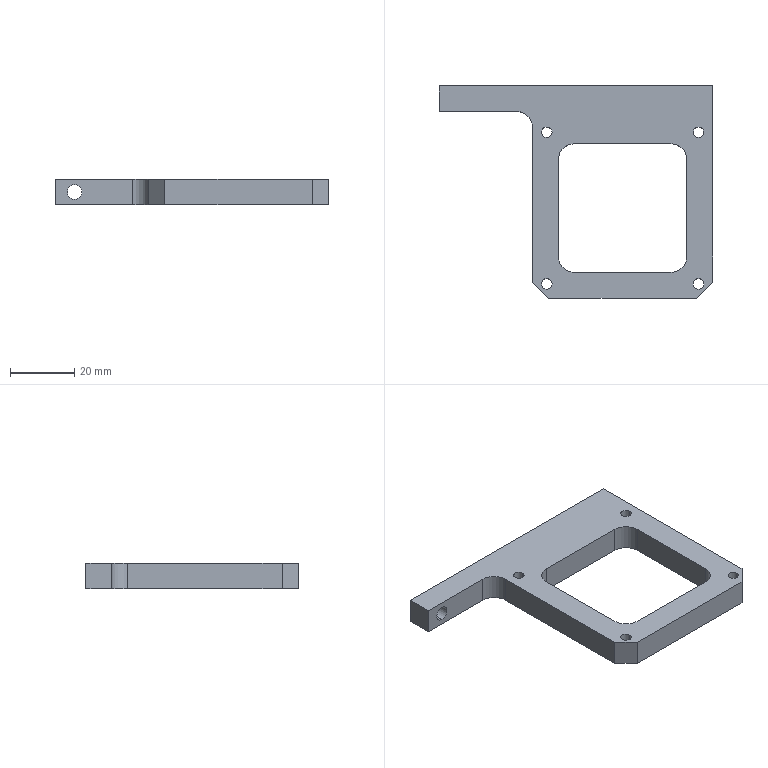Part | SolidWorks | features BaseBody 1 | 1 solid | 33 faces | box 85 x 66 x 8 mm | volume 18162 mm3 | cylinder 17 | plane 14 | cone 2 | commonest cylinder face diameters 3.242 x10 10 x5 4.5 x2
STEP:
#1=CARTESIAN_POINT('',(-10.691,18.57,0.));
#2=VERTEX_POINT('',#1);
#3=CARTESIAN_POINT('',(-7.449,18.57,0.));
#4=VERTEX_POINT('',#3);
#5=CARTESIAN_POINT('',(-9.07,18.57,0.));
#6=DIRECTION('',(0.,0.,1.));
#7=DIRECTION('',(1.,0.,0.));
#8=AXIS2_PLACEMENT_3D('',#5,#6,#7);
#9=CIRCLE('',#8,1.621);
#10=EDGE_CURVE('',#2,#4,#9,.T.);
#11=ORIENTED_EDGE('',*,*,#10,.F.);
#12=CARTESIAN_POINT('',(-10.691,18.57,8.));
#13=VERTEX_POINT('',#12);
#14=CARTESIAN_POINT('',(-10.691,18.57,-99.912));
#15=DIRECTION('',(0.,0.,1.));
#16=VECTOR('',#15,1000.);
#17=LINE('',#14,#16);
#18=EDGE_CURVE('',#2,#13,#17,.T.);
#19=ORIENTED_EDGE('',*,*,#18,.T.);
#20=CARTESIAN_POINT('',(-7.449,18.57,8.));
#21=VERTEX_POINT('',#20);
#22=CARTESIAN_POINT('',(-9.07,18.57,8.));
#23=DIRECTION('',(0.,0.,-1.));
#24=DIRECTION('',(1.,0.,0.));
#25=AXIS2_PLACEMENT_3D('',#22,#23,#24);
#26=CIRCLE('',#25,1.621);
#27=EDGE_CURVE('',#21,#13,#26,.T.);
#28=ORIENTED_EDGE('',*,*,#27,.F.);
#29=CARTESIAN_POINT('',(-7.449,18.57,-99.912));
#30=DIRECTION('',(0.,0.,1.));
#31=VECTOR('',#30,1000.);
#32=LINE('',#29,#31);
#33=EDGE_CURVE('',#4,#21,#32,.T.);
#34=ORIENTED_EDGE('',*,*,#33,.F.);
#35=EDGE_LOOP('',(#11,#19,#28,#34));
#36=FACE_OUTER_BOUND('',#35,.T.);
#37=CARTESIAN_POINT('',(-9.07,18.57,-99.912));
#38=DIRECTION('',(0.,0.,1.));
#39=DIRECTION('',(1.,0.,0.));
#40=AXIS2_PLACEMENT_3D('',#37,#38,#39);
#41=CYLINDRICAL_SURFACE('',#40,1.621);
#42=ADVANCED_FACE('',(#36),#41,.F.);
#43=CARTESIAN_POINT('',(36.449,18.57,0.));
#44=VERTEX_POINT('',#43);
#45=CARTESIAN_POINT('',(39.691,18.57,0.));
#46=VERTEX_POINT('',#45);
#47=CARTESIAN_POINT('',(38.07,18.57,0.));
#48=DIRECTION('',(0.,0.,1.));
#49=DIRECTION('',(1.,0.,0.));
#50=AXIS2_PLACEMENT_3D('',#47,#48,#49);
#51=CIRCLE('',#50,1.621);
#52=EDGE_CURVE('',#44,#46,#51,.T.);
#53=ORIENTED_EDGE('',*,*,#52,.F.);
#54=CARTESIAN_POINT('',(36.449,18.57,8.));
#55=VERTEX_POINT('',#54);
#56=CARTESIAN_POINT('',(36.449,18.57,-99.912));
#57=DIRECTION('',(0.,0.,1.));
#58=VECTOR('',#57,1000.);
#59=LINE('',#56,#58);
#60=EDGE_CURVE('',#44,#55,#59,.T.);
#61=ORIENTED_EDGE('',*,*,#60,.T.);
#62=CARTESIAN_POINT('',(39.691,18.57,8.));
#63=VERTEX_POINT('',#62);
#64=CARTESIAN_POINT('',(38.07,18.57,8.));
#65=DIRECTION('',(0.,0.,-1.));
#66=DIRECTION('',(1.,0.,0.));
#67=AXIS2_PLACEMENT_3D('',#64,#65,#66);
#68=CIRCLE('',#67,1.621);
#69=EDGE_CURVE('',#63,#55,#68,.T.);
#70=ORIENTED_EDGE('',*,*,#69,.F.);
#71=CARTESIAN_POINT('',(39.691,18.57,-99.912));
#72=DIRECTION('',(0.,0.,1.));
#73=VECTOR('',#72,1000.);
#74=LINE('',#71,#73);
#75=EDGE_CURVE('',#46,#63,#74,.T.);
#76=ORIENTED_EDGE('',*,*,#75,.F.);
#77=EDGE_LOOP('',(#53,#61,#70,#76));
#78=FACE_OUTER_BOUND('',#77,.T.);
#79=CARTESIAN_POINT('',(38.07,18.57,-99.912));
#80=DIRECTION('',(0.,0.,1.));
#81=DIRECTION('',(1.,0.,0.));
#82=AXIS2_PLACEMENT_3D('',#79,#80,#81);
#83=CYLINDRICAL_SURFACE('',#82,1.621);
#84=ADVANCED_FACE('',(#78),#83,.F.);
#85=CARTESIAN_POINT('',(36.449,-28.57,0.));
#86=VERTEX_POINT('',#85);
#87=CARTESIAN_POINT('',(39.691,-28.57,0.));
#88=VERTEX_POINT('',#87);
#89=CARTESIAN_POINT('',(38.07,-28.57,0.));
#90=DIRECTION('',(0.,0.,1.));
#91=DIRECTION('',(1.,0.,0.));
#92=AXIS2_PLACEMENT_3D('',#89,#90,#91);
#93=CIRCLE('',#92,1.621);
#94=EDGE_CURVE('',#86,#88,#93,.T.);
#95=ORIENTED_EDGE('',*,*,#94,.F.);
#96=CARTESIAN_POINT('',(36.449,-28.57,8.));
#97=VERTEX_POINT('',#96);
#98=CARTESIAN_POINT('',(36.449,-28.57,-99.912));
#99=DIRECTION('',(0.,0.,1.));
#100=VECTOR('',#99,1000.);
#101=LINE('',#98,#100);
#102=EDGE_CURVE('',#86,#97,#101,.T.);
#103=ORIENTED_EDGE('',*,*,#102,.T.);
#104=CARTESIAN_POINT('',(39.691,-28.57,8.));
#105=VERTEX_POINT('',#104);
#106=CARTESIAN_POINT('',(38.07,-28.57,8.));
#107=DIRECTION('',(0.,0.,-1.));
#108=DIRECTION('',(1.,0.,0.));
#109=AXIS2_PLACEMENT_3D('',#106,#107,#108);
#110=CIRCLE('',#109,1.621);
#111=EDGE_CURVE('',#105,#97,#110,.T.);
#112=ORIENTED_EDGE('',*,*,#111,.F.);
#113=CARTESIAN_POINT('',(39.691,-28.57,-99.912));
#114=DIRECTION('',(0.,0.,1.));
#115=VECTOR('',#114,1000.);
#116=LINE('',#113,#115);
#117=EDGE_CURVE('',#88,#105,#116,.T.);
#118=ORIENTED_EDGE('',*,*,#117,.F.);
#119=EDGE_LOOP('',(#95,#103,#112,#118));
#120=FACE_OUTER_BOUND('',#119,.T.);
#121=CARTESIAN_POINT('',(38.07,-28.57,-99.912));
#122=DIRECTION('',(0.,0.,1.));
#123=DIRECTION('',(1.,0.,0.));
#124=AXIS2_PLACEMENT_3D('',#121,#122,#123);
#125=CYLINDRICAL_SURFACE('',#124,1.621);
#126=ADVANCED_FACE('',(#120),#125,.F.);
#127=CARTESIAN_POINT('',(-10.691,-28.57,0.));
#128=VERTEX_POINT('',#127);
#129=CARTESIAN_POINT('',(-7.449,-28.57,0.));
#130=VERTEX_POINT('',#129);
#131=CARTESIAN_POINT('',(-9.07,-28.57,0.));
#132=DIRECTION('',(0.,0.,1.));
#133=DIRECTION('',(1.,0.,0.));
#134=AXIS2_PLACEMENT_3D('',#131,#132,#133);
#135=CIRCLE('',#134,1.621);
#136=EDGE_CURVE('',#128,#130,#135,.T.);
#137=ORIENTED_EDGE('',*,*,#136,.F.);
#138=CARTESIAN_POINT('',(-10.691,-28.57,8.));
#139=VERTEX_POINT('',#138);
#140=CARTESIAN_POINT('',(-10.691,-28.57,-99.912));
#141=DIRECTION('',(0.,0.,1.));
#142=VECTOR('',#141,1000.);
#143=LINE('',#140,#142);
#144=EDGE_CURVE('',#128,#139,#143,.T.);
#145=ORIENTED_EDGE('',*,*,#144,.T.);
#146=CARTESIAN_POINT('',(-7.449,-28.57,8.));
#147=VERTEX_POINT('',#146);
#148=CARTESIAN_POINT('',(-9.07,-28.57,8.));
#149=DIRECTION('',(0.,0.,-1.));
#150=DIRECTION('',(1.,0.,0.));
#151=AXIS2_PLACEMENT_3D('',#148,#149,#150);
#152=CIRCLE('',#151,1.621);
#153=EDGE_CURVE('',#147,#139,#152,.T.);
#154=ORIENTED_EDGE('',*,*,#153,.F.);
#155=CARTESIAN_POINT('',(-7.449,-28.57,-99.912));
#156=DIRECTION('',(0.,0.,1.));
#157=VECTOR('',#156,1000.);
#158=LINE('',#155,#157);
#159=EDGE_CURVE('',#130,#147,#158,.T.);
#160=ORIENTED_EDGE('',*,*,#159,.F.);
#161=EDGE_LOOP('',(#137,#145,#154,#160));
#162=FACE_OUTER_BOUND('',#161,.T.);
#163=CARTESIAN_POINT('',(-9.07,-28.57,-99.912));
#164=DIRECTION('',(0.,0.,1.));
#165=DIRECTION('',(1.,0.,0.));
#166=AXIS2_PLACEMENT_3D('',#163,#164,#165);
#167=CYLINDRICAL_SURFACE('',#166,1.621);
#168=ADVANCED_FACE('',(#162),#167,.F.);
#169=CARTESIAN_POINT('',(-36.495,33.,6.25));
#170=VERTEX_POINT('',#169);
#171=CARTESIAN_POINT('',(-36.495,33.,1.75));
#172=VERTEX_POINT('',#171);
#173=CARTESIAN_POINT('',(-36.495,33.,4.));
#174=DIRECTION('',(0.,-1.,0.));
#175=DIRECTION('',(0.,0.,-1.));
#176=AXIS2_PLACEMENT_3D('',#173,#174,#175);
#177=CIRCLE('',#176,2.25);
#178=EDGE_CURVE('',#170,#172,#177,.T.);
#179=ORIENTED_EDGE('',*,*,#178,.F.);
#180=CARTESIAN_POINT('',(-36.495,25.,6.25));
#181=VERTEX_POINT('',#180);
#182=CARTESIAN_POINT('',(-36.495,132.912,6.25));
#183=DIRECTION('',(0.,-1.,0.));
#184=VECTOR('',#183,1000.);
#185=LINE('',#182,#184);
#186=EDGE_CURVE('',#170,#181,#185,.T.);
#187=ORIENTED_EDGE('',*,*,#186,.T.);
#188=CARTESIAN_POINT('',(-36.495,25.,1.75));
#189=VERTEX_POINT('',#188);
#190=CARTESIAN_POINT('',(-36.495,25.,4.));
#191=DIRECTION('',(0.,1.,0.));
#192=DIRECTION('',(0.,0.,-1.));
#193=AXIS2_PLACEMENT_3D('',#190,#191,#192);
#194=CIRCLE('',#193,2.25);
#195=EDGE_CURVE('',#189,#181,#194,.T.);
#196=ORIENTED_EDGE('',*,*,#195,.F.);
#197=CARTESIAN_POINT('',(-36.495,132.912,1.75));
#198=DIRECTION('',(0.,-1.,0.));
#199=VECTOR('',#198,1000.);
#200=LINE('',#197,#199);
#201=EDGE_CURVE('',#172,#189,#200,.T.);
#202=ORIENTED_EDGE('',*,*,#201,.F.);
#203=EDGE_LOOP('',(#179,#187,#196,#202));
#204=FACE_OUTER_BOUND('',#203,.T.);
#205=CARTESIAN_POINT('',(-36.495,132.912,4.));
#206=DIRECTION('',(0.,-1.,0.));
#207=DIRECTION('',(0.,0.,-1.));
#208=AXIS2_PLACEMENT_3D('',#205,#206,#207);
#209=CYLINDRICAL_SURFACE('',#208,2.25);
#210=ADVANCED_FACE('',(#204),#209,.F.);
#211=CARTESIAN_POINT('',(16.126,23.,4.));
#212=VERTEX_POINT('',#211);
#213=CARTESIAN_POINT('',(14.505,23.,2.379));
#214=VERTEX_POINT('',#213);
#215=CARTESIAN_POINT('',(14.505,23.,4.));
#216=DIRECTION('',(0.,1.,0.));
#217=DIRECTION('',(-1.,0.,0.));
#218=AXIS2_PLACEMENT_3D('',#215,#216,#217);
#219=CIRCLE('',#218,1.621);
#220=EDGE_CURVE('',#212,#214,#219,.T.);
#221=ORIENTED_EDGE('',*,*,#220,.F.);
#222=CARTESIAN_POINT('',(16.126,33.,4.));
#223=VERTEX_POINT('',#222);
#224=CARTESIAN_POINT('',(16.126,28.,4.));
#225=DIRECTION('',(0.,1.,0.));
#226=VECTOR('',#225,1000.);
#227=LINE('',#224,#226);
#228=EDGE_CURVE('',#212,#223,#227,.T.);
#229=ORIENTED_EDGE('',*,*,#228,.T.);
#230=CARTESIAN_POINT('',(12.884,33.,4.));
#231=VERTEX_POINT('',#230);
#232=CARTESIAN_POINT('',(14.505,33.,4.));
#233=DIRECTION('',(0.,-1.,0.));
#234=DIRECTION('',(-1.,0.,0.));
#235=AXIS2_PLACEMENT_3D('',#232,#233,#234);
#236=CIRCLE('',#235,1.621);
#237=EDGE_CURVE('',#231,#223,#236,.T.);
#238=ORIENTED_EDGE('',*,*,#237,.F.);
#239=CARTESIAN_POINT('',(12.884,23.,4.));
#240=VERTEX_POINT('',#239);
#241=CARTESIAN_POINT('',(12.884,28.,4.));
#242=DIRECTION('',(0.,1.,0.));
#243=VECTOR('',#242,1000.);
#244=LINE('',#241,#243);
#245=EDGE_CURVE('',#240,#231,#244,.T.);
#246=ORIENTED_EDGE('',*,*,#245,.F.);
#247=CARTESIAN_POINT('',(14.505,23.,4.));
#248=DIRECTION('',(0.,1.,0.));
#249=DIRECTION('',(-1.,0.,0.));
#250=AXIS2_PLACEMENT_3D('',#247,#248,#249);
#251=CIRCLE('',#250,1.621);
#252=EDGE_CURVE('',#214,#240,#251,.T.);
#253=ORIENTED_EDGE('',*,*,#252,.F.);
#254=EDGE_LOOP('',(#221,#229,#238,#246,#253));
#255=FACE_OUTER_BOUND('',#254,.T.);
#256=CARTESIAN_POINT('',(14.505,28.,4.));
#257=DIRECTION('',(0.,1.,0.));
#258=DIRECTION('',(-1.,0.,0.));
#259=AXIS2_PLACEMENT_3D('',#256,#257,#258);
#260=CYLINDRICAL_SURFACE('',#259,1.621);
#261=ADVANCED_FACE('',(#255),#260,.F.);
#262=CARTESIAN_POINT('',(14.505,22.026,4.));
#263=VERTEX_POINT('',#262);
#264=CARTESIAN_POINT('',(14.505,23.,5.621));
#265=VERTEX_POINT('',#264);
#266=CARTESIAN_POINT('',(14.505,23.,5.621));
#267=DIRECTION('',(0.,0.515,0.8572));
#268=VECTOR('',#267,1000.);
#269=LINE('',#266,#268);
#270=EDGE_CURVE('',#263,#265,#269,.T.);
#271=ORIENTED_EDGE('',*,*,#270,.F.);
#272=CARTESIAN_POINT('',(14.505,23.,2.379));
#273=DIRECTION('',(0.,0.515,-0.8572));
#274=VECTOR('',#273,1000.);
#275=LINE('',#272,#274);
#276=EDGE_CURVE('',#263,#214,#275,.T.);
#277=ORIENTED_EDGE('',*,*,#276,.T.);
#278=ORIENTED_EDGE('',*,*,#252,.T.);
#279=CARTESIAN_POINT('',(14.505,23.,4.));
#280=DIRECTION('',(0.,1.,0.));
#281=DIRECTION('',(-1.,0.,0.));
#282=AXIS2_PLACEMENT_3D('',#279,#280,#281);
#283=CIRCLE('',#282,1.621);
#284=EDGE_CURVE('',#240,#265,#283,.T.);
#285=ORIENTED_EDGE('',*,*,#284,.T.);
#286=EDGE_LOOP('',(#271,#277,#278,#285));
#287=FACE_OUTER_BOUND('',#286,.T.);
#288=CARTESIAN_POINT('',(14.505,23.,4.));
#289=DIRECTION('',(0.,1.,0.));
#290=DIRECTION('',(0.,0.,1.));
#291=AXIS2_PLACEMENT_3D('',#288,#289,#290);
#292=CONICAL_SURFACE('',#291,1.621,1.03);
#293=ADVANCED_FACE('',(#287),#292,.F.);
#294=CARTESIAN_POINT('',(29.5,-25.,8.));
#295=VERTEX_POINT('',#294);
#296=CARTESIAN_POINT('',(-0.5,-25.,8.));
#297=VERTEX_POINT('',#296);
#298=CARTESIAN_POINT('',(5.57,-25.,8.));
#299=DIRECTION('',(-1.,0.,0.));
#300=VECTOR('',#299,1000.);
#301=LINE('',#298,#300);
#302=EDGE_CURVE('',#295,#297,#301,.T.);
#303=ORIENTED_EDGE('',*,*,#302,.T.);
#304=CARTESIAN_POINT('',(-5.5,-20.,8.));
#305=VERTEX_POINT('',#304);
#306=CARTESIAN_POINT('',(-0.5,-20.,8.));
#307=DIRECTION('',(0.,0.,-1.));
#308=DIRECTION('',(-1.,0.,0.));
#309=AXIS2_PLACEMENT_3D('',#306,#307,#308);
#310=CIRCLE('',#309,5.);
#311=EDGE_CURVE('',#297,#305,#310,.T.);
#312=ORIENTED_EDGE('',*,*,#311,.T.);
#313=CARTESIAN_POINT('',(-5.5,10.,8.));
#314=VERTEX_POINT('',#313);
#315=CARTESIAN_POINT('',(-5.5,5.57,8.));
#316=DIRECTION('',(0.,1.,0.));
#317=VECTOR('',#316,1000.);
#318=LINE('',#315,#317);
#319=EDGE_CURVE('',#305,#314,#318,.T.);
#320=ORIENTED_EDGE('',*,*,#319,.T.);
#321=CARTESIAN_POINT('',(-0.5,15.,8.));
#322=VERTEX_POINT('',#321);
#323=CARTESIAN_POINT('',(-0.5,10.,8.));
#324=DIRECTION('',(0.,0.,-1.));
#325=DIRECTION('',(-1.,0.,0.));
#326=AXIS2_PLACEMENT_3D('',#323,#324,#325);
#327=CIRCLE('',#326,5.);
#328=EDGE_CURVE('',#314,#322,#327,.T.);
#329=ORIENTED_EDGE('',*,*,#328,.T.);
#330=CARTESIAN_POINT('',(29.5,15.,8.));
#331=VERTEX_POINT('',#330);
#332=CARTESIAN_POINT('',(5.57,15.,8.));
#333=DIRECTION('',(1.,0.,0.));
#334=VECTOR('',#333,1000.);
#335=LINE('',#332,#334);
#336=EDGE_CURVE('',#322,#331,#335,.T.);
#337=ORIENTED_EDGE('',*,*,#336,.T.);
#338=CARTESIAN_POINT('',(34.5,10.,8.));
#339=VERTEX_POINT('',#338);
#340=CARTESIAN_POINT('',(29.5,10.,8.));
#341=DIRECTION('',(0.,0.,-1.));
#342=DIRECTION('',(-1.,0.,0.));
#343=AXIS2_PLACEMENT_3D('',#340,#341,#342);
#344=CIRCLE('',#343,5.);
#345=EDGE_CURVE('',#331,#339,#344,.T.);
#346=ORIENTED_EDGE('',*,*,#345,.T.);
#347=CARTESIAN_POINT('',(34.5,-20.,8.));
#348=VERTEX_POINT('',#347);
#349=CARTESIAN_POINT('',(34.5,5.57,8.));
#350=DIRECTION('',(0.,-1.,0.));
#351=VECTOR('',#350,1000.);
#352=LINE('',#349,#351);
#353=EDGE_CURVE('',#339,#348,#352,.T.);
#354=ORIENTED_EDGE('',*,*,#353,.T.);
#355=CARTESIAN_POINT('',(29.5,-20.,8.));
#356=DIRECTION('',(0.,0.,-1.));
#357=DIRECTION('',(-1.,0.,0.));
#358=AXIS2_PLACEMENT_3D('',#355,#356,#357);
#359=CIRCLE('',#358,5.);
#360=EDGE_CURVE('',#348,#295,#359,.T.);
#361=ORIENTED_EDGE('',*,*,#360,.T.);
#362=EDGE_LOOP('',(#303,#312,#320,#329,#337,#346,#354,#361));
#363=FACE_BOUND('',#362,.T.);
#364=ORIENTED_EDGE('',*,*,#27,.T.);
#365=CARTESIAN_POINT('',(-9.07,18.57,8.));
#366=DIRECTION('',(0.,0.,-1.));
#367=DIRECTION('',(1.,0.,0.));
#368=AXIS2_PLACEMENT_3D('',#365,#366,#367);
#369=CIRCLE('',#368,1.621);
#370=EDGE_CURVE('',#13,#21,#369,.T.);
#371=ORIENTED_EDGE('',*,*,#370,.T.);
#372=EDGE_LOOP('',(#364,#371));
#373=FACE_BOUND('',#372,.T.);
#374=ORIENTED_EDGE('',*,*,#69,.T.);
#375=CARTESIAN_POINT('',(38.07,18.57,8.));
#376=DIRECTION('',(0.,0.,-1.));
#377=DIRECTION('',(1.,0.,0.));
#378=AXIS2_PLACEMENT_3D('',#375,#376,#377);
#379=CIRCLE('',#378,1.621);
#380=EDGE_CURVE('',#55,#63,#379,.T.);
#381=ORIENTED_EDGE('',*,*,#380,.T.);
#382=EDGE_LOOP('',(#374,#381));
#383=FACE_BOUND('',#382,.T.);
#384=ORIENTED_EDGE('',*,*,#111,.T.);
#385=CARTESIAN_POINT('',(38.07,-28.57,8.));
#386=DIRECTION('',(0.,0.,-1.));
#387=DIRECTION('',(1.,0.,0.));
#388=AXIS2_PLACEMENT_3D('',#385,#386,#387);
#389=CIRCLE('',#388,1.621);
#390=EDGE_CURVE('',#97,#105,#389,.T.);
#391=ORIENTED_EDGE('',*,*,#390,.T.);
#392=EDGE_LOOP('',(#384,#391));
#393=FACE_BOUND('',#392,.T.);
#394=ORIENTED_EDGE('',*,*,#153,.T.);
#395=CARTESIAN_POINT('',(-9.07,-28.57,8.));
#396=DIRECTION('',(0.,0.,-1.));
#397=DIRECTION('',(1.,0.,0.));
#398=AXIS2_PLACEMENT_3D('',#395,#396,#397);
#399=CIRCLE('',#398,1.621);
#400=EDGE_CURVE('',#139,#147,#399,.T.);
#401=ORIENTED_EDGE('',*,*,#400,.T.);
#402=EDGE_LOOP('',(#394,#401));
#403=FACE_BOUND('',#402,.T.);
#404=CARTESIAN_POINT('',(-13.5,-28.,8.));
#405=VERTEX_POINT('',#404);
#406=CARTESIAN_POINT('',(-8.5,-33.,8.));
#407=VERTEX_POINT('',#406);
#408=CARTESIAN_POINT('',(-13.5,-28.,8.));
#409=DIRECTION('',(0.7071,-0.7071,0.));
#410=VECTOR('',#409,1000.);
#411=LINE('',#408,#410);
#412=EDGE_CURVE('',#405,#407,#411,.T.);
#413=ORIENTED_EDGE('',*,*,#412,.T.);
#414=CARTESIAN_POINT('',(37.5,-33.,8.));
#415=VERTEX_POINT('',#414);
#416=CARTESIAN_POINT('',(5.57,-33.,8.));
#417=DIRECTION('',(1.,0.,0.));
#418=VECTOR('',#417,1000.);
#419=LINE('',#416,#418);
#420=EDGE_CURVE('',#407,#415,#419,.T.);
#421=ORIENTED_EDGE('',*,*,#420,.T.);
#422=CARTESIAN_POINT('',(42.5,-28.,8.));
#423=VERTEX_POINT('',#422);
#424=CARTESIAN_POINT('',(37.5,-33.,8.));
#425=DIRECTION('',(0.7071,0.7071,0.));
#426=VECTOR('',#425,1000.);
#427=LINE('',#424,#426);
#428=EDGE_CURVE('',#415,#423,#427,.T.);
#429=ORIENTED_EDGE('',*,*,#428,.T.);
#430=CARTESIAN_POINT('',(42.5,33.,8.));
#431=VERTEX_POINT('',#430);
#432=CARTESIAN_POINT('',(42.5,5.57,8.));
#433=DIRECTION('',(0.,1.,0.));
#434=VECTOR('',#433,1000.);
#435=LINE('',#432,#434);
#436=EDGE_CURVE('',#423,#431,#435,.T.);
#437=ORIENTED_EDGE('',*,*,#436,.T.);
#438=CARTESIAN_POINT('',(-42.5,33.,8.));
#439=VERTEX_POINT('',#438);
#440=CARTESIAN_POINT('',(5.57,33.,8.));
#441=DIRECTION('',(-1.,0.,0.));
#442=VECTOR('',#441,1000.);
#443=LINE('',#440,#442);
#444=EDGE_CURVE('',#431,#439,#443,.T.);
#445=ORIENTED_EDGE('',*,*,#444,.T.);
#446=CARTESIAN_POINT('',(-42.5,25.,8.));
#447=VERTEX_POINT('',#446);
#448=CARTESIAN_POINT('',(-42.5,5.57,8.));
#449=DIRECTION('',(0.,-1.,0.));
#450=VECTOR('',#449,1000.);
#451=LINE('',#448,#450);
#452=EDGE_CURVE('',#439,#447,#451,.T.);
#453=ORIENTED_EDGE('',*,*,#452,.T.);
#454=CARTESIAN_POINT('',(-18.5,25.,8.));
#455=VERTEX_POINT('',#454);
#456=CARTESIAN_POINT('',(5.57,25.,8.));
#457=DIRECTION('',(1.,0.,0.));
#458=VECTOR('',#457,1000.);
#459=LINE('',#456,#458);
#460=EDGE_CURVE('',#447,#455,#459,.T.);
#461=ORIENTED_EDGE('',*,*,#460,.T.);
#462=CARTESIAN_POINT('',(-13.5,20.,8.));
#463=VERTEX_POINT('',#462);
#464=CARTESIAN_POINT('',(-18.5,20.,8.));
#465=DIRECTION('',(0.,0.,-1.));
#466=DIRECTION('',(1.,0.,0.));
#467=AXIS2_PLACEMENT_3D('',#464,#465,#466);
#468=CIRCLE('',#467,5.);
#469=EDGE_CURVE('',#455,#463,#468,.T.);
#470=ORIENTED_EDGE('',*,*,#469,.T.);
#471=CARTESIAN_POINT('',(-13.5,5.57,8.));
#472=DIRECTION('',(0.,-1.,0.));
#473=VECTOR('',#472,1000.);
#474=LINE('',#471,#473);
#475=EDGE_CURVE('',#463,#405,#474,.T.);
#476=ORIENTED_EDGE('',*,*,#475,.T.);
#477=EDGE_LOOP('',(#413,#421,#429,#437,#445,#453,#461,#470,#476));
#478=FACE_OUTER_BOUND('',#477,.T.);
#479=CARTESIAN_POINT('',(5.57,5.57,8.));
#480=DIRECTION('',(0.,0.,1.));
#481=DIRECTION('',(1.,0.,0.));
#482=AXIS2_PLACEMENT_3D('',#479,#480,#481);
#483=PLANE('',#482);
#484=ADVANCED_FACE('',(#363,#373,#383,#393,#403,#478),#483,.T.);
#485=CARTESIAN_POINT('',(-0.5,-25.,0.));
#486=VERTEX_POINT('',#485);
#487=CARTESIAN_POINT('',(-0.5,-25.,8.));
#488=DIRECTION('',(0.,0.,1.));
#489=VECTOR('',#488,1000.);
#490=LINE('',#487,#489);
#491=EDGE_CURVE('',#486,#297,#490,.T.);
#492=ORIENTED_EDGE('',*,*,#491,.F.);
#493=CARTESIAN_POINT('',(-5.5,-20.,0.));
#494=VERTEX_POINT('',#493);
#495=CARTESIAN_POINT('',(-0.5,-20.,0.));
#496=DIRECTION('',(0.,0.,1.));
#497=DIRECTION('',(-1.,0.,0.));
#498=AXIS2_PLACEMENT_3D('',#495,#496,#497);
#499=CIRCLE('',#498,5.);
#500=EDGE_CURVE('',#494,#486,#499,.T.);
#501=ORIENTED_EDGE('',*,*,#500,.F.);
#502=CARTESIAN_POINT('',(-5.5,-20.,8.));
#503=DIRECTION('',(0.,0.,-1.));
#504=VECTOR('',#503,1000.);
#505=LINE('',#502,#504);
#506=EDGE_CURVE('',#305,#494,#505,.T.);
#507=ORIENTED_EDGE('',*,*,#506,.F.);
#508=ORIENTED_EDGE('',*,*,#311,.F.);
#509=EDGE_LOOP('',(#492,#501,#507,#508));
#510=FACE_OUTER_BOUND('',#509,.T.);
#511=CARTESIAN_POINT('',(-0.5,-20.,8.));
#512=DIRECTION('',(0.,0.,-1.));
#513=DIRECTION('',(-1.,0.,0.));
#514=AXIS2_PLACEMENT_3D('',#511,#512,#513);
#515=CYLINDRICAL_SURFACE('',#514,5.);
#516=ADVANCED_FACE('',(#510),#515,.F.);
#517=ORIENTED_EDGE('',*,*,#302,.F.);
#518=CARTESIAN_POINT('',(29.5,-25.,0.));
#519=VERTEX_POINT('',#518);
#520=CARTESIAN_POINT('',(29.5,-25.,8.));
#521=DIRECTION('',(0.,0.,1.));
#522=VECTOR('',#521,1000.);
#523=LINE('',#520,#522);
#524=EDGE_CURVE('',#519,#295,#523,.T.);
#525=ORIENTED_EDGE('',*,*,#524,.F.);
#526=CARTESIAN_POINT('',(-5.5,-25.,0.));
#527=DIRECTION('',(1.,0.,0.));
#528=VECTOR('',#527,1000.);
#529=LINE('',#526,#528);
#530=EDGE_CURVE('',#486,#519,#529,.T.);
#531=ORIENTED_EDGE('',*,*,#530,.F.);
#532=ORIENTED_EDGE('',*,*,#491,.T.);
#533=EDGE_LOOP('',(#517,#525,#531,#532));
#534=FACE_OUTER_BOUND('',#533,.T.);
#535=CARTESIAN_POINT('',(-5.5,-25.,8.));
#536=DIRECTION('',(0.,-1.,0.));
#537=DIRECTION('',(0.,0.,-1.));
#538=AXIS2_PLACEMENT_3D('',#535,#536,#537);
#539=PLANE('',#538);
#540=ADVANCED_FACE('',(#534),#539,.F.);
#541=CARTESIAN_POINT('',(34.5,-20.,0.));
#542=VERTEX_POINT('',#541);
#543=CARTESIAN_POINT('',(34.5,-20.,8.));
#544=DIRECTION('',(0.,0.,1.));
#545=VECTOR('',#544,1000.);
#546=LINE('',#543,#545);
#547=EDGE_CURVE('',#542,#348,#546,.T.);
#548=ORIENTED_EDGE('',*,*,#547,.F.);
#549=CARTESIAN_POINT('',(29.5,-20.,0.));
#550=DIRECTION('',(0.,0.,1.));
#551=DIRECTION('',(-1.,0.,0.));
#552=AXIS2_PLACEMENT_3D('',#549,#550,#551);
#553=CIRCLE('',#552,5.);
#554=EDGE_CURVE('',#519,#542,#553,.T.);
#555=ORIENTED_EDGE('',*,*,#554,.F.);
#556=ORIENTED_EDGE('',*,*,#524,.T.);
#557=ORIENTED_EDGE('',*,*,#360,.F.);
#558=EDGE_LOOP('',(#548,#555,#556,#557));
#559=FACE_OUTER_BOUND('',#558,.T.);
#560=CARTESIAN_POINT('',(29.5,-20.,8.));
#561=DIRECTION('',(0.,0.,-1.));
#562=DIRECTION('',(-1.,0.,0.));
#563=AXIS2_PLACEMENT_3D('',#560,#561,#562);
#564=CYLINDRICAL_SURFACE('',#563,5.);
#565=ADVANCED_FACE('',(#559),#564,.F.);
#566=ORIENTED_EDGE('',*,*,#353,.F.);
#567=CARTESIAN_POINT('',(34.5,10.,0.));
#568=VERTEX_POINT('',#567);
#569=CARTESIAN_POINT('',(34.5,10.,8.));
#570=DIRECTION('',(0.,0.,1.));
#571=VECTOR('',#570,1000.);
#572=LINE('',#569,#571);
#573=EDGE_CURVE('',#568,#339,#572,.T.);
#574=ORIENTED_EDGE('',*,*,#573,.F.);
#575=CARTESIAN_POINT('',(34.5,-25.,0.));
#576=DIRECTION('',(0.,1.,0.));
#577=VECTOR('',#576,1000.);
#578=LINE('',#575,#577);
#579=EDGE_CURVE('',#542,#568,#578,.T.);
#580=ORIENTED_EDGE('',*,*,#579,.F.);
#581=ORIENTED_EDGE('',*,*,#547,.T.);
#582=EDGE_LOOP('',(#566,#574,#580,#581));
#583=FACE_OUTER_BOUND('',#582,.T.);
#584=CARTESIAN_POINT('',(34.5,-25.,8.));
#585=DIRECTION('',(1.,0.,0.));
#586=DIRECTION('',(0.,0.,-1.));
#587=AXIS2_PLACEMENT_3D('',#584,#585,#586);
#588=PLANE('',#587);
#589=ADVANCED_FACE('',(#583),#588,.F.);
#590=CARTESIAN_POINT('',(29.5,15.,0.));
#591=VERTEX_POINT('',#590);
#592=CARTESIAN_POINT('',(29.5,15.,8.));
#593=DIRECTION('',(0.,0.,1.));
#594=VECTOR('',#593,1000.);
#595=LINE('',#592,#594);
#596=EDGE_CURVE('',#591,#331,#595,.T.);
#597=ORIENTED_EDGE('',*,*,#596,.F.);
#598=CARTESIAN_POINT('',(29.5,10.,0.));
#599=DIRECTION('',(0.,0.,1.));
#600=DIRECTION('',(-1.,0.,0.));
#601=AXIS2_PLACEMENT_3D('',#598,#599,#600);
#602=CIRCLE('',#601,5.);
#603=EDGE_CURVE('',#568,#591,#602,.T.);
#604=ORIENTED_EDGE('',*,*,#603,.F.);
#605=ORIENTED_EDGE('',*,*,#573,.T.);
#606=ORIENTED_EDGE('',*,*,#345,.F.);
#607=EDGE_LOOP('',(#597,#604,#605,#606));
#608=FACE_OUTER_BOUND('',#607,.T.);
#609=CARTESIAN_POINT('',(29.5,10.,8.));
#610=DIRECTION('',(0.,0.,-1.));
#611=DIRECTION('',(-1.,0.,0.));
#612=AXIS2_PLACEMENT_3D('',#609,#610,#611);
#613=CYLINDRICAL_SURFACE('',#612,5.);
#614=ADVANCED_FACE('',(#608),#613,.F.);
#615=ORIENTED_EDGE('',*,*,#336,.F.);
#616=CARTESIAN_POINT('',(-0.5,15.,0.));
#617=VERTEX_POINT('',#616);
#618=CARTESIAN_POINT('',(-0.5,15.,8.));
#619=DIRECTION('',(0.,0.,1.));
#620=VECTOR('',#619,1000.);
#621=LINE('',#618,#620);
#622=EDGE_CURVE('',#617,#322,#621,.T.);
#623=ORIENTED_EDGE('',*,*,#622,.F.);
#624=CARTESIAN_POINT('',(34.5,15.,0.));
#625=DIRECTION('',(-1.,0.,0.));
#626=VECTOR('',#625,1000.);
#627=LINE('',#624,#626);
#628=EDGE_CURVE('',#591,#617,#627,.T.);
#629=ORIENTED_EDGE('',*,*,#628,.F.);
#630=ORIENTED_EDGE('',*,*,#596,.T.);
#631=EDGE_LOOP('',(#615,#623,#629,#630));
#632=FACE_OUTER_BOUND('',#631,.T.);
#633=CARTESIAN_POINT('',(34.5,15.,8.));
#634=DIRECTION('',(0.,1.,0.));
#635=DIRECTION('',(0.,0.,1.));
#636=AXIS2_PLACEMENT_3D('',#633,#634,#635);
#637=PLANE('',#636);
#638=ADVANCED_FACE('',(#632),#637,.F.);
#639=CARTESIAN_POINT('',(-5.5,10.,0.));
#640=VERTEX_POINT('',#639);
#641=CARTESIAN_POINT('',(-5.5,10.,8.));
#642=DIRECTION('',(0.,0.,1.));
#643=VECTOR('',#642,1000.);
#644=LINE('',#641,#643);
#645=EDGE_CURVE('',#640,#314,#644,.T.);
#646=ORIENTED_EDGE('',*,*,#645,.F.);
#647=CARTESIAN_POINT('',(-0.5,10.,0.));
#648=DIRECTION('',(0.,0.,1.));
#649=DIRECTION('',(-1.,0.,0.));
#650=AXIS2_PLACEMENT_3D('',#647,#648,#649);
#651=CIRCLE('',#650,5.);
#652=EDGE_CURVE('',#617,#640,#651,.T.);
#653=ORIENTED_EDGE('',*,*,#652,.F.);
#654=ORIENTED_EDGE('',*,*,#622,.T.);
#655=ORIENTED_EDGE('',*,*,#328,.F.);
#656=EDGE_LOOP('',(#646,#653,#654,#655));
#657=FACE_OUTER_BOUND('',#656,.T.);
#658=CARTESIAN_POINT('',(-0.5,10.,8.));
#659=DIRECTION('',(0.,0.,-1.));
#660=DIRECTION('',(-1.,0.,0.));
#661=AXIS2_PLACEMENT_3D('',#658,#659,#660);
#662=CYLINDRICAL_SURFACE('',#661,5.);
#663=ADVANCED_FACE('',(#657),#662,.F.);
#664=CARTESIAN_POINT('',(-5.5,15.,0.));
#665=DIRECTION('',(0.,-1.,0.));
#666=VECTOR('',#665,1000.);
#667=LINE('',#664,#666);
#668=EDGE_CURVE('',#640,#494,#667,.T.);
#669=ORIENTED_EDGE('',*,*,#668,.F.);
#670=ORIENTED_EDGE('',*,*,#645,.T.);
#671=ORIENTED_EDGE('',*,*,#319,.F.);
#672=ORIENTED_EDGE('',*,*,#506,.T.);
#673=EDGE_LOOP('',(#669,#670,#671,#672));
#674=FACE_OUTER_BOUND('',#673,.T.);
#675=CARTESIAN_POINT('',(-5.5,15.,8.));
#676=DIRECTION('',(-1.,0.,0.));
#677=DIRECTION('',(0.,0.,1.));
#678=AXIS2_PLACEMENT_3D('',#675,#676,#677);
#679=PLANE('',#678);
#680=ADVANCED_FACE('',(#674),#679,.F.);
#681=ORIENTED_EDGE('',*,*,#18,.F.);
#682=CARTESIAN_POINT('',(-9.07,18.57,0.));
#683=DIRECTION('',(0.,0.,1.));
#684=DIRECTION('',(1.,0.,0.));
#685=AXIS2_PLACEMENT_3D('',#682,#683,#684);
#686=CIRCLE('',#685,1.621);
#687=EDGE_CURVE('',#4,#2,#686,.T.);
#688=ORIENTED_EDGE('',*,*,#687,.F.);
#689=ORIENTED_EDGE('',*,*,#33,.T.);
#690=ORIENTED_EDGE('',*,*,#370,.F.);
#691=EDGE_LOOP('',(#681,#688,#689,#690));
#692=FACE_OUTER_BOUND('',#691,.T.);
#693=CARTESIAN_POINT('',(-9.07,18.57,-99.912));
#694=DIRECTION('',(0.,0.,1.));
#695=DIRECTION('',(1.,0.,0.));
#696=AXIS2_PLACEMENT_3D('',#693,#694,#695);
#697=CYLINDRICAL_SURFACE('',#696,1.621);
#698=ADVANCED_FACE('',(#692),#697,.F.);
#699=ORIENTED_EDGE('',*,*,#60,.F.);
#700=CARTESIAN_POINT('',(38.07,18.57,0.));
#701=DIRECTION('',(0.,0.,1.));
#702=DIRECTION('',(1.,0.,0.));
#703=AXIS2_PLACEMENT_3D('',#700,#701,#702);
#704=CIRCLE('',#703,1.621);
#705=EDGE_CURVE('',#46,#44,#704,.T.);
#706=ORIENTED_EDGE('',*,*,#705,.F.);
#707=ORIENTED_EDGE('',*,*,#75,.T.);
#708=ORIENTED_EDGE('',*,*,#380,.F.);
#709=EDGE_LOOP('',(#699,#706,#707,#708));
#710=FACE_OUTER_BOUND('',#709,.T.);
#711=CARTESIAN_POINT('',(38.07,18.57,-99.912));
#712=DIRECTION('',(0.,0.,1.));
#713=DIRECTION('',(1.,0.,0.));
#714=AXIS2_PLACEMENT_3D('',#711,#712,#713);
#715=CYLINDRICAL_SURFACE('',#714,1.621);
#716=ADVANCED_FACE('',(#710),#715,.F.);
#717=ORIENTED_EDGE('',*,*,#102,.F.);
#718=CARTESIAN_POINT('',(38.07,-28.57,0.));
#719=DIRECTION('',(0.,0.,1.));
#720=DIRECTION('',(1.,0.,0.));
#721=AXIS2_PLACEMENT_3D('',#718,#719,#720);
#722=CIRCLE('',#721,1.621);
#723=EDGE_CURVE('',#88,#86,#722,.T.);
#724=ORIENTED_EDGE('',*,*,#723,.F.);
#725=ORIENTED_EDGE('',*,*,#117,.T.);
#726=ORIENTED_EDGE('',*,*,#390,.F.);
#727=EDGE_LOOP('',(#717,#724,#725,#726));
#728=FACE_OUTER_BOUND('',#727,.T.);
#729=CARTESIAN_POINT('',(38.07,-28.57,-99.912));
#730=DIRECTION('',(0.,0.,1.));
#731=DIRECTION('',(1.,0.,0.));
#732=AXIS2_PLACEMENT_3D('',#729,#730,#731);
#733=CYLINDRICAL_SURFACE('',#732,1.621);
#734=ADVANCED_FACE('',(#728),#733,.F.);
#735=ORIENTED_EDGE('',*,*,#144,.F.);
#736=CARTESIAN_POINT('',(-9.07,-28.57,0.));
#737=DIRECTION('',(0.,0.,1.));
#738=DIRECTION('',(1.,0.,0.));
#739=AXIS2_PLACEMENT_3D('',#736,#737,#738);
#740=CIRCLE('',#739,1.621);
#741=EDGE_CURVE('',#130,#128,#740,.T.);
#742=ORIENTED_EDGE('',*,*,#741,.F.);
#743=ORIENTED_EDGE('',*,*,#159,.T.);
#744=ORIENTED_EDGE('',*,*,#400,.F.);
#745=EDGE_LOOP('',(#735,#742,#743,#744));
#746=FACE_OUTER_BOUND('',#745,.T.);
#747=CARTESIAN_POINT('',(-9.07,-28.57,-99.912));
#748=DIRECTION('',(0.,0.,1.));
#749=DIRECTION('',(1.,0.,0.));
#750=AXIS2_PLACEMENT_3D('',#747,#748,#749);
#751=CYLINDRICAL_SURFACE('',#750,1.621);
#752=ADVANCED_FACE('',(#746),#751,.F.);
#753=CARTESIAN_POINT('',(-8.5,-33.,0.));
#754=VERTEX_POINT('',#753);
#755=CARTESIAN_POINT('',(-8.5,-33.,0.));
#756=DIRECTION('',(0.,0.,-1.));
#757=VECTOR('',#756,1000.);
#758=LINE('',#755,#757);
#759=EDGE_CURVE('',#407,#754,#758,.T.);
#760=ORIENTED_EDGE('',*,*,#759,.T.);
#761=CARTESIAN_POINT('',(37.5,-33.,0.));
#762=VERTEX_POINT('',#761);
#763=CARTESIAN_POINT('',(42.5,-33.,0.));
#764=DIRECTION('',(1.,0.,0.));
#765=VECTOR('',#764,1000.);
#766=LINE('',#763,#765);
#767=EDGE_CURVE('',#754,#762,#766,.T.);
#768=ORIENTED_EDGE('',*,*,#767,.T.);
#769=CARTESIAN_POINT('',(37.5,-33.,0.));
#770=DIRECTION('',(0.,0.,1.));
#771=VECTOR('',#770,1000.);
#772=LINE('',#769,#771);
#773=EDGE_CURVE('',#762,#415,#772,.T.);
#774=ORIENTED_EDGE('',*,*,#773,.T.);
#775=ORIENTED_EDGE('',*,*,#420,.F.);
#776=EDGE_LOOP('',(#760,#768,#774,#775));
#777=FACE_OUTER_BOUND('',#776,.T.);
#778=CARTESIAN_POINT('',(42.5,-33.,0.));
#779=DIRECTION('',(0.,-1.,0.));
#780=DIRECTION('',(0.,0.,-1.));
#781=AXIS2_PLACEMENT_3D('',#778,#779,#780);
#782=PLANE('',#781);
#783=ADVANCED_FACE('',(#777),#782,.T.);
#784=CARTESIAN_POINT('',(-13.5,-28.,0.));
#785=VERTEX_POINT('',#784);
#786=CARTESIAN_POINT('',(-11.,-30.5,0.));
#787=DIRECTION('',(0.7071,-0.7071,0.));
#788=VECTOR('',#787,1000.);
#789=LINE('',#786,#788);
#790=EDGE_CURVE('',#785,#754,#789,.T.);
#791=ORIENTED_EDGE('',*,*,#790,.T.);
#792=ORIENTED_EDGE('',*,*,#759,.F.);
#793=ORIENTED_EDGE('',*,*,#412,.F.);
#794=CARTESIAN_POINT('',(-13.5,-28.,0.));
#795=DIRECTION('',(0.,0.,-1.));
#796=VECTOR('',#795,1000.);
#797=LINE('',#794,#796);
#798=EDGE_CURVE('',#405,#785,#797,.T.);
#799=ORIENTED_EDGE('',*,*,#798,.T.);
#800=EDGE_LOOP('',(#791,#792,#793,#799));
#801=FACE_OUTER_BOUND('',#800,.T.);
#802=CARTESIAN_POINT('',(-11.,-30.5,0.));
#803=DIRECTION('',(-0.7071,-0.7071,0.));
#804=DIRECTION('',(0.7071,-0.7071,0.));
#805=AXIS2_PLACEMENT_3D('',#802,#803,#804);
#806=PLANE('',#805);
#807=ADVANCED_FACE('',(#801),#806,.T.);
#808=CARTESIAN_POINT('',(-13.5,20.,0.));
#809=VERTEX_POINT('',#808);
#810=CARTESIAN_POINT('',(-13.5,20.,0.));
#811=DIRECTION('',(0.,0.,-1.));
#812=VECTOR('',#811,1000.);
#813=LINE('',#810,#812);
#814=EDGE_CURVE('',#463,#809,#813,.T.);
#815=ORIENTED_EDGE('',*,*,#814,.T.);
#816=CARTESIAN_POINT('',(-13.5,-33.,0.));
#817=DIRECTION('',(0.,-1.,0.));
#818=VECTOR('',#817,1000.);
#819=LINE('',#816,#818);
#820=EDGE_CURVE('',#809,#785,#819,.T.);
#821=ORIENTED_EDGE('',*,*,#820,.T.);
#822=ORIENTED_EDGE('',*,*,#798,.F.);
#823=ORIENTED_EDGE('',*,*,#475,.F.);
#824=EDGE_LOOP('',(#815,#821,#822,#823));
#825=FACE_OUTER_BOUND('',#824,.T.);
#826=CARTESIAN_POINT('',(-13.5,-33.,0.));
#827=DIRECTION('',(-1.,0.,0.));
#828=DIRECTION('',(0.,0.,1.));
#829=AXIS2_PLACEMENT_3D('',#826,#827,#828);
#830=PLANE('',#829);
#831=ADVANCED_FACE('',(#825),#830,.T.);
#832=ORIENTED_EDGE('',*,*,#814,.F.);
#833=ORIENTED_EDGE('',*,*,#469,.F.);
#834=CARTESIAN_POINT('',(-18.5,25.,0.));
#835=VERTEX_POINT('',#834);
#836=CARTESIAN_POINT('',(-18.5,25.,0.));
#837=DIRECTION('',(0.,0.,1.));
#838=VECTOR('',#837,1000.);
#839=LINE('',#836,#838);
#840=EDGE_CURVE('',#835,#455,#839,.T.);
#841=ORIENTED_EDGE('',*,*,#840,.F.);
#842=CARTESIAN_POINT('',(-18.5,20.,0.));
#843=DIRECTION('',(0.,0.,1.));
#844=DIRECTION('',(1.,0.,0.));
#845=AXIS2_PLACEMENT_3D('',#842,#843,#844);
#846=CIRCLE('',#845,5.);
#847=EDGE_CURVE('',#809,#835,#846,.T.);
#848=ORIENTED_EDGE('',*,*,#847,.F.);
#849=EDGE_LOOP('',(#832,#833,#841,#848));
#850=FACE_OUTER_BOUND('',#849,.T.);
#851=CARTESIAN_POINT('',(-18.5,20.,0.));
#852=DIRECTION('',(0.,0.,1.));
#853=DIRECTION('',(1.,0.,0.));
#854=AXIS2_PLACEMENT_3D('',#851,#852,#853);
#855=CYLINDRICAL_SURFACE('',#854,5.);
#856=ADVANCED_FACE('',(#850),#855,.F.);
#857=ORIENTED_EDGE('',*,*,#195,.T.);
#858=CARTESIAN_POINT('',(-36.495,25.,4.));
#859=DIRECTION('',(0.,1.,0.));
#860=DIRECTION('',(0.,0.,-1.));
#861=AXIS2_PLACEMENT_3D('',#858,#859,#860);
#862=CIRCLE('',#861,2.25);
#863=EDGE_CURVE('',#181,#189,#862,.T.);
#864=ORIENTED_EDGE('',*,*,#863,.T.);
#865=EDGE_LOOP('',(#857,#864));
#866=FACE_BOUND('',#865,.T.);
#867=CARTESIAN_POINT('',(-42.5,25.,0.));
#868=VERTEX_POINT('',#867);
#869=CARTESIAN_POINT('',(-42.5,25.,0.));
#870=DIRECTION('',(0.,0.,-1.));
#871=VECTOR('',#870,1000.);
#872=LINE('',#869,#871);
#873=EDGE_CURVE('',#447,#868,#872,.T.);
#874=ORIENTED_EDGE('',*,*,#873,.T.);
#875=CARTESIAN_POINT('',(-13.5,25.,0.));
#876=DIRECTION('',(1.,0.,0.));
#877=VECTOR('',#876,1000.);
#878=LINE('',#875,#877);
#879=EDGE_CURVE('',#868,#835,#878,.T.);
#880=ORIENTED_EDGE('',*,*,#879,.T.);
#881=ORIENTED_EDGE('',*,*,#840,.T.);
#882=ORIENTED_EDGE('',*,*,#460,.F.);
#883=EDGE_LOOP('',(#874,#880,#881,#882));
#884=FACE_OUTER_BOUND('',#883,.T.);
#885=CARTESIAN_POINT('',(-13.5,25.,0.));
#886=DIRECTION('',(0.,-1.,0.));
#887=DIRECTION('',(0.,0.,-1.));
#888=AXIS2_PLACEMENT_3D('',#885,#886,#887);
#889=PLANE('',#888);
#890=ADVANCED_FACE('',(#866,#884),#889,.T.);
#891=CARTESIAN_POINT('',(-42.5,33.,0.));
#892=VERTEX_POINT('',#891);
#893=CARTESIAN_POINT('',(-42.5,25.,0.));
#894=DIRECTION('',(0.,-1.,0.));
#895=VECTOR('',#894,1000.);
#896=LINE('',#893,#895);
#897=EDGE_CURVE('',#892,#868,#896,.T.);
#898=ORIENTED_EDGE('',*,*,#897,.T.);
#899=ORIENTED_EDGE('',*,*,#873,.F.);
#900=ORIENTED_EDGE('',*,*,#452,.F.);
#901=CARTESIAN_POINT('',(-42.5,33.,0.));
#902=DIRECTION('',(0.,0.,-1.));
#903=VECTOR('',#902,1000.);
#904=LINE('',#901,#903);
#905=EDGE_CURVE('',#439,#892,#904,.T.);
#906=ORIENTED_EDGE('',*,*,#905,.T.);
#907=EDGE_LOOP('',(#898,#899,#900,#906));
#908=FACE_OUTER_BOUND('',#907,.T.);
#909=CARTESIAN_POINT('',(-42.5,25.,0.));
#910=DIRECTION('',(-1.,0.,0.));
#911=DIRECTION('',(0.,0.,1.));
#912=AXIS2_PLACEMENT_3D('',#909,#910,#911);
#913=PLANE('',#912);
#914=ADVANCED_FACE('',(#908),#913,.T.);
#915=CARTESIAN_POINT('',(-36.495,33.,4.));
#916=DIRECTION('',(0.,-1.,0.));
#917=DIRECTION('',(0.,0.,-1.));
#918=AXIS2_PLACEMENT_3D('',#915,#916,#917);
#919=CIRCLE('',#918,2.25);
#920=EDGE_CURVE('',#172,#170,#919,.T.);
#921=ORIENTED_EDGE('',*,*,#920,.T.);
#922=ORIENTED_EDGE('',*,*,#178,.T.);
#923=EDGE_LOOP('',(#921,#922));
#924=FACE_BOUND('',#923,.T.);
#925=ORIENTED_EDGE('',*,*,#237,.T.);
#926=CARTESIAN_POINT('',(14.505,33.,4.));
#927=DIRECTION('',(0.,-1.,0.));
#928=DIRECTION('',(-1.,0.,0.));
#929=AXIS2_PLACEMENT_3D('',#926,#927,#928);
#930=CIRCLE('',#929,1.621);
#931=EDGE_CURVE('',#223,#231,#930,.T.);
#932=ORIENTED_EDGE('',*,*,#931,.T.);
#933=EDGE_LOOP('',(#925,#932));
#934=FACE_BOUND('',#933,.T.);
#935=CARTESIAN_POINT('',(42.5,33.,0.));
#936=VERTEX_POINT('',#935);
#937=CARTESIAN_POINT('',(-42.5,33.,0.));
#938=DIRECTION('',(-1.,0.,0.));
#939=VECTOR('',#938,1000.);
#940=LINE('',#937,#939);
#941=EDGE_CURVE('',#936,#892,#940,.T.);
#942=ORIENTED_EDGE('',*,*,#941,.T.);
#943=ORIENTED_EDGE('',*,*,#905,.F.);
#944=ORIENTED_EDGE('',*,*,#444,.F.);
#945=CARTESIAN_POINT('',(42.5,33.,0.));
#946=DIRECTION('',(0.,0.,-1.));
#947=VECTOR('',#946,1000.);
#948=LINE('',#945,#947);
#949=EDGE_CURVE('',#431,#936,#948,.T.);
#950=ORIENTED_EDGE('',*,*,#949,.T.);
#951=EDGE_LOOP('',(#942,#943,#944,#950));
#952=FACE_OUTER_BOUND('',#951,.T.);
#953=CARTESIAN_POINT('',(-42.5,33.,0.));
#954=DIRECTION('',(0.,1.,0.));
#955=DIRECTION('',(0.,0.,1.));
#956=AXIS2_PLACEMENT_3D('',#953,#954,#955);
#957=PLANE('',#956);
#958=ADVANCED_FACE('',(#924,#934,#952),#957,.T.);
#959=ORIENTED_EDGE('',*,*,#949,.F.);
#960=ORIENTED_EDGE('',*,*,#436,.F.);
#961=CARTESIAN_POINT('',(42.5,-28.,0.));
#962=VERTEX_POINT('',#961);
#963=CARTESIAN_POINT('',(42.5,-28.,0.));
#964=DIRECTION('',(0.,0.,-1.));
#965=VECTOR('',#964,1000.);
#966=LINE('',#963,#965);
#967=EDGE_CURVE('',#423,#962,#966,.T.);
#968=ORIENTED_EDGE('',*,*,#967,.T.);
#969=CARTESIAN_POINT('',(42.5,33.,0.));
#970=DIRECTION('',(0.,1.,0.));
#971=VECTOR('',#970,1000.);
#972=LINE('',#969,#971);
#973=EDGE_CURVE('',#962,#936,#972,.T.);
#974=ORIENTED_EDGE('',*,*,#973,.T.);
#975=EDGE_LOOP('',(#959,#960,#968,#974));
#976=FACE_OUTER_BOUND('',#975,.T.);
#977=CARTESIAN_POINT('',(42.5,33.,0.));
#978=DIRECTION('',(1.,0.,0.));
#979=DIRECTION('',(0.,0.,-1.));
#980=AXIS2_PLACEMENT_3D('',#977,#978,#979);
#981=PLANE('',#980);
#982=ADVANCED_FACE('',(#976),#981,.T.);
#983=CARTESIAN_POINT('',(40.,-30.5,0.));
#984=DIRECTION('',(0.7071,0.7071,0.));
#985=VECTOR('',#984,1000.);
#986=LINE('',#983,#985);
#987=EDGE_CURVE('',#762,#962,#986,.T.);
#988=ORIENTED_EDGE('',*,*,#987,.T.);
#989=ORIENTED_EDGE('',*,*,#967,.F.);
#990=ORIENTED_EDGE('',*,*,#428,.F.);
#991=ORIENTED_EDGE('',*,*,#773,.F.);
#992=EDGE_LOOP('',(#988,#989,#990,#991));
#993=FACE_OUTER_BOUND('',#992,.T.);
#994=CARTESIAN_POINT('',(40.,-30.5,0.));
#995=DIRECTION('',(0.7071,-0.7071,0.));
#996=DIRECTION('',(0.7071,0.7071,0.));
#997=AXIS2_PLACEMENT_3D('',#994,#995,#996);
#998=PLANE('',#997);
#999=ADVANCED_FACE('',(#993),#998,.T.);
#1000=ORIENTED_EDGE('',*,*,#500,.T.);
#1001=ORIENTED_EDGE('',*,*,#530,.T.);
#1002=ORIENTED_EDGE('',*,*,#554,.T.);
#1003=ORIENTED_EDGE('',*,*,#579,.T.);
#1004=ORIENTED_EDGE('',*,*,#603,.T.);
#1005=ORIENTED_EDGE('',*,*,#628,.T.);
#1006=ORIENTED_EDGE('',*,*,#652,.T.);
#1007=ORIENTED_EDGE('',*,*,#668,.T.);
#1008=EDGE_LOOP('',(#1000,#1001,#1002,#1003,#1004,#1005,#1006,#1007));
#1009=FACE_BOUND('',#1008,.T.);
#1010=ORIENTED_EDGE('',*,*,#687,.T.);
#1011=ORIENTED_EDGE('',*,*,#10,.T.);
#1012=EDGE_LOOP('',(#1010,#1011));
#1013=FACE_BOUND('',#1012,.T.);
#1014=ORIENTED_EDGE('',*,*,#705,.T.);
#1015=ORIENTED_EDGE('',*,*,#52,.T.);
#1016=EDGE_LOOP('',(#1014,#1015));
#1017=FACE_BOUND('',#1016,.T.);
#1018=ORIENTED_EDGE('',*,*,#723,.T.);
#1019=ORIENTED_EDGE('',*,*,#94,.T.);
#1020=EDGE_LOOP('',(#1018,#1019));
#1021=FACE_BOUND('',#1020,.T.);
#1022=ORIENTED_EDGE('',*,*,#741,.T.);
#1023=ORIENTED_EDGE('',*,*,#136,.T.);
#1024=EDGE_LOOP('',(#1022,#1023));
#1025=FACE_BOUND('',#1024,.T.);
#1026=ORIENTED_EDGE('',*,*,#767,.F.);
#1027=ORIENTED_EDGE('',*,*,#790,.F.);
#1028=ORIENTED_EDGE('',*,*,#820,.F.);
#1029=ORIENTED_EDGE('',*,*,#847,.T.);
#1030=ORIENTED_EDGE('',*,*,#879,.F.);
#1031=ORIENTED_EDGE('',*,*,#897,.F.);
#1032=ORIENTED_EDGE('',*,*,#941,.F.);
#1033=ORIENTED_EDGE('',*,*,#973,.F.);
#1034=ORIENTED_EDGE('',*,*,#987,.F.);
#1035=EDGE_LOOP('',(#1026,#1027,#1028,#1029,#1030,#1031,#1032,#1033,#1034));
#1036=FACE_OUTER_BOUND('',#1035,.T.);
#1037=CARTESIAN_POINT('',(5.57,5.57,0.));
#1038=DIRECTION('',(0.,0.,1.));
#1039=DIRECTION('',(1.,0.,0.));
#1040=AXIS2_PLACEMENT_3D('',#1037,#1038,#1039);
#1041=PLANE('',#1040);
#1042=ADVANCED_FACE('',(#1009,#1013,#1017,#1021,#1025,#1036),#1041,.F.);
#1043=ORIENTED_EDGE('',*,*,#186,.F.);
#1044=ORIENTED_EDGE('',*,*,#920,.F.);
#1045=ORIENTED_EDGE('',*,*,#201,.T.);
#1046=ORIENTED_EDGE('',*,*,#863,.F.);
#1047=EDGE_LOOP('',(#1043,#1044,#1045,#1046));
#1048=FACE_OUTER_BOUND('',#1047,.T.);
#1049=CARTESIAN_POINT('',(-36.495,132.912,4.));
#1050=DIRECTION('',(0.,-1.,0.));
#1051=DIRECTION('',(0.,0.,-1.));
#1052=AXIS2_PLACEMENT_3D('',#1049,#1050,#1051);
#1053=CYLINDRICAL_SURFACE('',#1052,2.25);
#1054=ADVANCED_FACE('',(#1048),#1053,.F.);
#1055=ORIENTED_EDGE('',*,*,#228,.F.);
#1056=CARTESIAN_POINT('',(14.505,23.,4.));
#1057=DIRECTION('',(0.,1.,0.));
#1058=DIRECTION('',(-1.,0.,0.));
#1059=AXIS2_PLACEMENT_3D('',#1056,#1057,#1058);
#1060=CIRCLE('',#1059,1.621);
#1061=EDGE_CURVE('',#265,#212,#1060,.T.);
#1062=ORIENTED_EDGE('',*,*,#1061,.F.);
#1063=ORIENTED_EDGE('',*,*,#284,.F.);
#1064=ORIENTED_EDGE('',*,*,#245,.T.);
#1065=ORIENTED_EDGE('',*,*,#931,.F.);
#1066=EDGE_LOOP('',(#1055,#1062,#1063,#1064,#1065));
#1067=FACE_OUTER_BOUND('',#1066,.T.);
#1068=CARTESIAN_POINT('',(14.505,28.,4.));
#1069=DIRECTION('',(0.,1.,0.));
#1070=DIRECTION('',(-1.,0.,0.));
#1071=AXIS2_PLACEMENT_3D('',#1068,#1069,#1070);
#1072=CYLINDRICAL_SURFACE('',#1071,1.621);
#1073=ADVANCED_FACE('',(#1067),#1072,.F.);
#1074=ORIENTED_EDGE('',*,*,#276,.F.);
#1075=ORIENTED_EDGE('',*,*,#270,.T.);
#1076=ORIENTED_EDGE('',*,*,#1061,.T.);
#1077=ORIENTED_EDGE('',*,*,#220,.T.);
#1078=EDGE_LOOP('',(#1074,#1075,#1076,#1077));
#1079=FACE_OUTER_BOUND('',#1078,.T.);
#1080=CARTESIAN_POINT('',(14.505,23.,4.));
#1081=DIRECTION('',(0.,1.,0.));
#1082=DIRECTION('',(0.,0.,1.));
#1083=AXIS2_PLACEMENT_3D('',#1080,#1081,#1082);
#1084=CONICAL_SURFACE('',#1083,1.621,1.03);
#1085=ADVANCED_FACE('',(#1079),#1084,.F.);
#1086=CLOSED_SHELL('',(#42,#84,#126,#168,#210,#261,#293,#484,#516,#540,#565,#589,#614,#638,#663,#680,#698,#716,#734,#752,#783,#807,#831,#856,#890,#914,#958,#982,#999,#1042,#1054,#1073,#1085));
#1087=MANIFOLD_SOLID_BREP('',#1086);
#1088=CARTESIAN_POINT('',(0.,0.,0.));
#1089=DIRECTION('',(0.,0.,1.));
#1090=DIRECTION('',(1.,0.,0.));
#1091=AXIS2_PLACEMENT_3D('',#1088,#1089,#1090);
#1092=(LENGTH_UNIT()NAMED_UNIT(*)SI_UNIT(.MILLI.,.METRE.));
#1093=UNCERTAINTY_MEASURE_WITH_UNIT(LENGTH_MEASURE(0.00001),#1092,'','');
#1094=(NAMED_UNIT(*)PLANE_ANGLE_UNIT()SI_UNIT($,.RADIAN.));
#1095=(NAMED_UNIT(*)SI_UNIT($,.STERADIAN.)SOLID_ANGLE_UNIT());
#1096=(GEOMETRIC_REPRESENTATION_CONTEXT(3)GLOBAL_UNCERTAINTY_ASSIGNED_CONTEXT((#1093))GLOBAL_UNIT_ASSIGNED_CONTEXT((#1092,#1094,#1095))REPRESENTATION_CONTEXT('',''));
#1097=ADVANCED_BREP_SHAPE_REPRESENTATION('',(#1087,#1091),#1096);